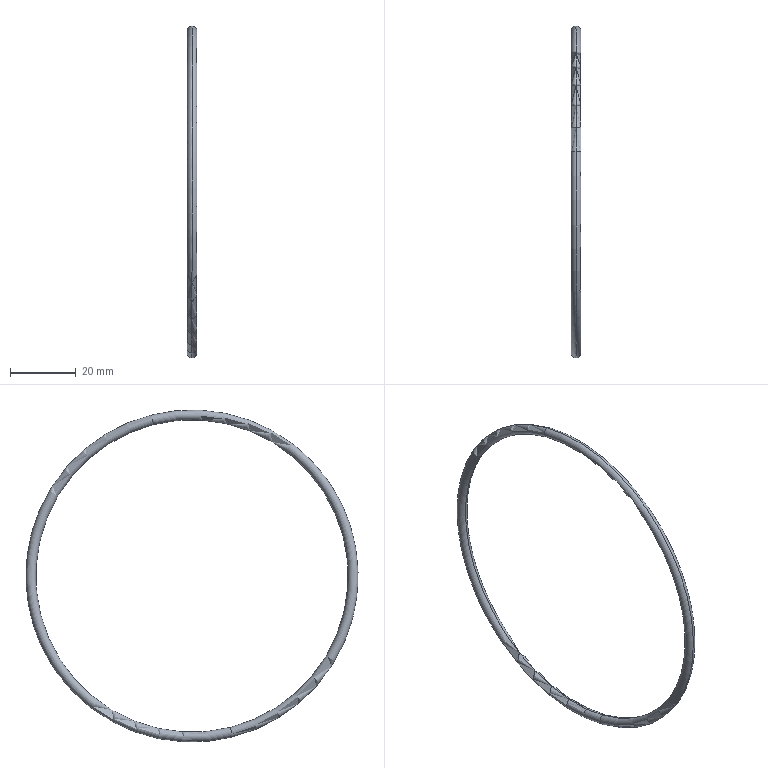Part | SolidWorks | features BaseBody 1 | 1 solid | 4 faces | box 3 x 101 x 101 mm | volume 2176 mm3 | torus 4
STEP:
#1=CARTESIAN_POINT('',(-1.,-12.359,-48.964));
#2=VERTEX_POINT('',#1);
#3=CARTESIAN_POINT('',(-1.,-11.625,-46.055));
#4=VERTEX_POINT('',#3);
#5=CARTESIAN_POINT('',(-1.,-11.992,-47.51));
#6=DIRECTION('',(0.,-0.9696,0.2447));
#7=DIRECTION('',(0.,-0.2447,-0.9696));
#8=AXIS2_PLACEMENT_3D('',#5,#6,#7);
#9=CIRCLE('',#8,1.5);
#10=EDGE_CURVE('',#2,#4,#9,.T.);
#11=ORIENTED_EDGE('',*,*,#10,.F.);
#12=CARTESIAN_POINT('',(-1.,12.359,48.964));
#13=VERTEX_POINT('',#12);
#14=CARTESIAN_POINT('',(-1.,0.,0.));
#15=DIRECTION('',(1.,0.,0.));
#16=DIRECTION('',(0.,0.,-1.));
#17=AXIS2_PLACEMENT_3D('',#14,#15,#16);
#18=CIRCLE('',#17,50.5);
#19=EDGE_CURVE('',#2,#13,#18,.T.);
#20=ORIENTED_EDGE('',*,*,#19,.T.);
#21=CARTESIAN_POINT('',(-1.,11.625,46.055));
#22=VERTEX_POINT('',#21);
#23=CARTESIAN_POINT('',(-1.,11.992,47.51));
#24=DIRECTION('',(0.,0.9696,-0.2447));
#25=DIRECTION('',(0.,0.2447,0.9696));
#26=AXIS2_PLACEMENT_3D('',#23,#24,#25);
#27=CIRCLE('',#26,1.5);
#28=EDGE_CURVE('',#13,#22,#27,.T.);
#29=ORIENTED_EDGE('',*,*,#28,.T.);
#30=CARTESIAN_POINT('',(-1.,0.,0.));
#31=DIRECTION('',(1.,0.,0.));
#32=DIRECTION('',(0.,0.,-1.));
#33=AXIS2_PLACEMENT_3D('',#30,#31,#32);
#34=CIRCLE('',#33,47.5);
#35=EDGE_CURVE('',#4,#22,#34,.T.);
#36=ORIENTED_EDGE('',*,*,#35,.F.);
#37=EDGE_LOOP('',(#11,#20,#29,#36));
#38=FACE_OUTER_BOUND('',#37,.T.);
#39=CARTESIAN_POINT('',(-1.,0.,0.));
#40=DIRECTION('',(1.,0.,0.));
#41=DIRECTION('',(0.,0.2447,0.9696));
#42=AXIS2_PLACEMENT_3D('',#39,#40,#41);
#43=TOROIDAL_SURFACE('',#42,49.,1.5);
#44=ADVANCED_FACE('',(#38),#43,.T.);
#45=ORIENTED_EDGE('',*,*,#28,.F.);
#46=CARTESIAN_POINT('',(-1.,0.,0.));
#47=DIRECTION('',(1.,0.,0.));
#48=DIRECTION('',(0.,0.,-1.));
#49=AXIS2_PLACEMENT_3D('',#46,#47,#48);
#50=CIRCLE('',#49,50.5);
#51=EDGE_CURVE('',#13,#2,#50,.T.);
#52=ORIENTED_EDGE('',*,*,#51,.T.);
#53=ORIENTED_EDGE('',*,*,#10,.T.);
#54=CARTESIAN_POINT('',(-1.,0.,0.));
#55=DIRECTION('',(1.,0.,0.));
#56=DIRECTION('',(0.,0.,-1.));
#57=AXIS2_PLACEMENT_3D('',#54,#55,#56);
#58=CIRCLE('',#57,47.5);
#59=EDGE_CURVE('',#22,#4,#58,.T.);
#60=ORIENTED_EDGE('',*,*,#59,.F.);
#61=EDGE_LOOP('',(#45,#52,#53,#60));
#62=FACE_OUTER_BOUND('',#61,.T.);
#63=CARTESIAN_POINT('',(-1.,0.,0.));
#64=DIRECTION('',(1.,0.,0.));
#65=DIRECTION('',(0.,0.2447,0.9696));
#66=AXIS2_PLACEMENT_3D('',#63,#64,#65);
#67=TOROIDAL_SURFACE('',#66,49.,1.5);
#68=ADVANCED_FACE('',(#62),#67,.T.);
#69=ORIENTED_EDGE('',*,*,#51,.F.);
#70=CARTESIAN_POINT('',(-1.,11.992,47.51));
#71=DIRECTION('',(0.,0.9696,-0.2447));
#72=DIRECTION('',(0.,0.2447,0.9696));
#73=AXIS2_PLACEMENT_3D('',#70,#71,#72);
#74=CIRCLE('',#73,1.5);
#75=EDGE_CURVE('',#22,#13,#74,.T.);
#76=ORIENTED_EDGE('',*,*,#75,.F.);
#77=ORIENTED_EDGE('',*,*,#59,.T.);
#78=CARTESIAN_POINT('',(-1.,-11.992,-47.51));
#79=DIRECTION('',(0.,-0.9696,0.2447));
#80=DIRECTION('',(0.,-0.2447,-0.9696));
#81=AXIS2_PLACEMENT_3D('',#78,#79,#80);
#82=CIRCLE('',#81,1.5);
#83=EDGE_CURVE('',#4,#2,#82,.T.);
#84=ORIENTED_EDGE('',*,*,#83,.T.);
#85=EDGE_LOOP('',(#69,#76,#77,#84));
#86=FACE_OUTER_BOUND('',#85,.T.);
#87=CARTESIAN_POINT('',(-1.,0.,0.));
#88=DIRECTION('',(1.,0.,0.));
#89=DIRECTION('',(0.,0.2447,0.9696));
#90=AXIS2_PLACEMENT_3D('',#87,#88,#89);
#91=TOROIDAL_SURFACE('',#90,49.,1.5);
#92=ADVANCED_FACE('',(#86),#91,.T.);
#93=ORIENTED_EDGE('',*,*,#19,.F.);
#94=ORIENTED_EDGE('',*,*,#83,.F.);
#95=ORIENTED_EDGE('',*,*,#35,.T.);
#96=ORIENTED_EDGE('',*,*,#75,.T.);
#97=EDGE_LOOP('',(#93,#94,#95,#96));
#98=FACE_OUTER_BOUND('',#97,.T.);
#99=CARTESIAN_POINT('',(-1.,0.,0.));
#100=DIRECTION('',(1.,0.,0.));
#101=DIRECTION('',(0.,0.2447,0.9696));
#102=AXIS2_PLACEMENT_3D('',#99,#100,#101);
#103=TOROIDAL_SURFACE('',#102,49.,1.5);
#104=ADVANCED_FACE('',(#98),#103,.T.);
#105=CLOSED_SHELL('',(#44,#68,#92,#104));
#106=MANIFOLD_SOLID_BREP('',#105);
#107=CARTESIAN_POINT('',(0.,0.,0.));
#108=DIRECTION('',(0.,0.,1.));
#109=DIRECTION('',(1.,0.,0.));
#110=AXIS2_PLACEMENT_3D('',#107,#108,#109);
#111=(LENGTH_UNIT()NAMED_UNIT(*)SI_UNIT(.MILLI.,.METRE.));
#112=UNCERTAINTY_MEASURE_WITH_UNIT(LENGTH_MEASURE(0.00001),#111,'','');
#113=(NAMED_UNIT(*)PLANE_ANGLE_UNIT()SI_UNIT($,.RADIAN.));
#114=(NAMED_UNIT(*)SI_UNIT($,.STERADIAN.)SOLID_ANGLE_UNIT());
#115=(GEOMETRIC_REPRESENTATION_CONTEXT(3)GLOBAL_UNCERTAINTY_ASSIGNED_CONTEXT((#112))GLOBAL_UNIT_ASSIGNED_CONTEXT((#111,#113,#114))REPRESENTATION_CONTEXT('',''));
#116=ADVANCED_BREP_SHAPE_REPRESENTATION('',(#106,#110),#115);